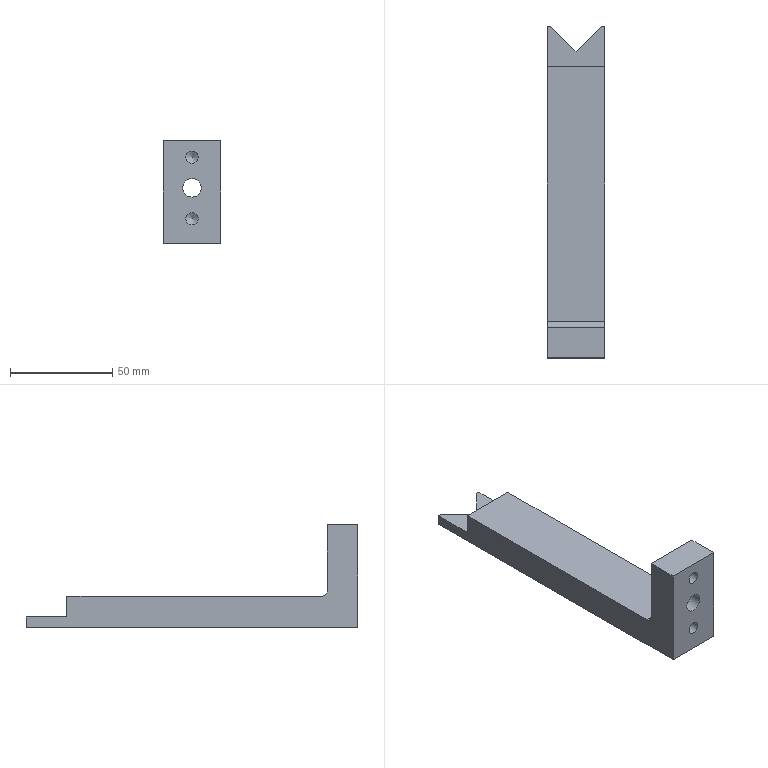Part | NX | features BREP 1 | 1 solid | 23 faces | box 28 x 162 x 50 mm | volume 74568 mm3 | plane 13 | cylinder 6 | cone 4 | commonest cylinder face diameters 6 x3 3.3 x2 9 x1
STEP:
#1=CARTESIAN_POINT('',(-14.,61.,7.5));
#2=VERTEX_POINT('',#1);
#3=CARTESIAN_POINT('',(-14.,-63.,7.5));
#4=VERTEX_POINT('',#3);
#5=CARTESIAN_POINT('',(-14.,-81.,7.5));
#6=DIRECTION('',(0.,-1.,0.));
#7=VECTOR('',#6,1000.);
#8=LINE('',#5,#7);
#9=EDGE_CURVE('',#2,#4,#8,.T.);
#10=ORIENTED_EDGE('',*,*,#9,.T.);
#11=CARTESIAN_POINT('',(14.,-63.,7.5));
#12=VERTEX_POINT('',#11);
#13=CARTESIAN_POINT('',(0.,-63.,7.5));
#14=DIRECTION('',(1.,0.,0.));
#15=VECTOR('',#14,1000.);
#16=LINE('',#13,#15);
#17=EDGE_CURVE('',#4,#12,#16,.T.);
#18=ORIENTED_EDGE('',*,*,#17,.T.);
#19=CARTESIAN_POINT('',(14.,61.,7.5));
#20=VERTEX_POINT('',#19);
#21=CARTESIAN_POINT('',(14.,-81.,7.5));
#22=DIRECTION('',(0.,1.,0.));
#23=VECTOR('',#22,1000.);
#24=LINE('',#21,#23);
#25=EDGE_CURVE('',#12,#20,#24,.T.);
#26=ORIENTED_EDGE('',*,*,#25,.T.);
#27=CARTESIAN_POINT('',(36.361,61.,7.5));
#28=DIRECTION('',(-1.,0.,0.));
#29=VECTOR('',#28,1000.);
#30=LINE('',#27,#29);
#31=EDGE_CURVE('',#20,#2,#30,.T.);
#32=ORIENTED_EDGE('',*,*,#31,.T.);
#33=EDGE_LOOP('',(#10,#18,#26,#32));
#34=FACE_BOUND('',#33,.T.);
#35=CARTESIAN_POINT('',(0.,0.,7.5));
#36=DIRECTION('',(0.,0.,-1.));
#37=DIRECTION('',(1.,0.,0.));
#38=AXIS2_PLACEMENT_3D('',#35,#36,#37);
#39=PLANE('',#38);
#40=ADVANCED_FACE('',(#34),#39,.F.);
#41=CARTESIAN_POINT('',(-14.,81.,-2.5));
#42=VERTEX_POINT('',#41);
#43=CARTESIAN_POINT('',(-14.,81.,-7.5));
#44=VERTEX_POINT('',#43);
#45=CARTESIAN_POINT('',(-14.,81.,7.5));
#46=DIRECTION('',(0.,0.,-1.));
#47=VECTOR('',#46,1000.);
#48=LINE('',#45,#47);
#49=EDGE_CURVE('',#42,#44,#48,.T.);
#50=ORIENTED_EDGE('',*,*,#49,.F.);
#51=CARTESIAN_POINT('',(-12.5,81.,-2.5));
#52=VERTEX_POINT('',#51);
#53=CARTESIAN_POINT('',(36.361,81.,-2.5));
#54=DIRECTION('',(-1.,0.,0.));
#55=VECTOR('',#54,1000.);
#56=LINE('',#53,#55);
#57=EDGE_CURVE('',#52,#42,#56,.T.);
#58=ORIENTED_EDGE('',*,*,#57,.F.);
#59=CARTESIAN_POINT('',(-12.5,81.,-7.5));
#60=VERTEX_POINT('',#59);
#61=CARTESIAN_POINT('',(-12.5,81.,35.451));
#62=DIRECTION('',(0.,0.,-1.));
#63=VECTOR('',#62,1000.);
#64=LINE('',#61,#63);
#65=EDGE_CURVE('',#52,#60,#64,.T.);
#66=ORIENTED_EDGE('',*,*,#65,.T.);
#67=CARTESIAN_POINT('',(-14.,81.,-7.5));
#68=DIRECTION('',(-1.,0.,0.));
#69=VECTOR('',#68,1000.);
#70=LINE('',#67,#69);
#71=EDGE_CURVE('',#60,#44,#70,.T.);
#72=ORIENTED_EDGE('',*,*,#71,.T.);
#73=EDGE_LOOP('',(#50,#58,#66,#72));
#74=FACE_BOUND('',#73,.T.);
#75=CARTESIAN_POINT('',(-14.,81.,7.5));
#76=DIRECTION('',(0.,-1.,0.));
#77=DIRECTION('',(0.,0.,1.));
#78=AXIS2_PLACEMENT_3D('',#75,#76,#77);
#79=PLANE('',#78);
#80=ADVANCED_FACE('',(#74),#79,.F.);
#81=CARTESIAN_POINT('',(14.,34.,-1.65));
#82=VERTEX_POINT('',#81);
#83=CARTESIAN_POINT('',(14.,34.,0.));
#84=DIRECTION('',(1.,0.,0.));
#85=DIRECTION('',(0.,0.,-1.));
#86=AXIS2_PLACEMENT_3D('',#83,#84,#85);
#87=CIRCLE('',#86,1.65);
#88=EDGE_CURVE('',#82,#82,#87,.T.);
#89=ORIENTED_EDGE('',*,*,#88,.F.);
#90=EDGE_LOOP('',(#89));
#91=FACE_BOUND('',#90,.T.);
#92=CARTESIAN_POINT('',(14.,24.,-1.65));
#93=VERTEX_POINT('',#92);
#94=CARTESIAN_POINT('',(14.,24.,0.));
#95=DIRECTION('',(1.,0.,0.));
#96=DIRECTION('',(0.,0.,-1.));
#97=AXIS2_PLACEMENT_3D('',#94,#95,#96);
#98=CIRCLE('',#97,1.65);
#99=EDGE_CURVE('',#93,#93,#98,.T.);
#100=ORIENTED_EDGE('',*,*,#99,.F.);
#101=EDGE_LOOP('',(#100));
#102=FACE_BOUND('',#101,.T.);
#103=CARTESIAN_POINT('',(14.,61.,-2.5));
#104=VERTEX_POINT('',#103);
#105=CARTESIAN_POINT('',(14.,81.,-2.5));
#106=VERTEX_POINT('',#105);
#107=CARTESIAN_POINT('',(14.,61.,-2.5));
#108=DIRECTION('',(0.,1.,0.));
#109=VECTOR('',#108,1000.);
#110=LINE('',#107,#109);
#111=EDGE_CURVE('',#104,#106,#110,.T.);
#112=ORIENTED_EDGE('',*,*,#111,.F.);
#113=CARTESIAN_POINT('',(14.,61.,7.5));
#114=DIRECTION('',(0.,0.,-1.));
#115=VECTOR('',#114,1000.);
#116=LINE('',#113,#115);
#117=EDGE_CURVE('',#20,#104,#116,.T.);
#118=ORIENTED_EDGE('',*,*,#117,.F.);
#119=ORIENTED_EDGE('',*,*,#25,.F.);
#120=CARTESIAN_POINT('',(14.,-66.,10.5));
#121=VERTEX_POINT('',#120);
#122=CARTESIAN_POINT('',(14.,-63.,10.5));
#123=DIRECTION('',(-1.,0.,0.));
#124=DIRECTION('',(0.,0.,1.));
#125=AXIS2_PLACEMENT_3D('',#122,#123,#124);
#126=CIRCLE('',#125,3.);
#127=EDGE_CURVE('',#12,#121,#126,.T.);
#128=ORIENTED_EDGE('',*,*,#127,.T.);
#129=CARTESIAN_POINT('',(14.,-66.,42.5));
#130=VERTEX_POINT('',#129);
#131=CARTESIAN_POINT('',(14.,-66.,7.5));
#132=DIRECTION('',(0.,0.,1.));
#133=VECTOR('',#132,1000.);
#134=LINE('',#131,#133);
#135=EDGE_CURVE('',#121,#130,#134,.T.);
#136=ORIENTED_EDGE('',*,*,#135,.T.);
#137=CARTESIAN_POINT('',(14.,-81.,42.5));
#138=VERTEX_POINT('',#137);
#139=CARTESIAN_POINT('',(14.,-81.,42.5));
#140=DIRECTION('',(0.,-1.,0.));
#141=VECTOR('',#140,1000.);
#142=LINE('',#139,#141);
#143=EDGE_CURVE('',#130,#138,#142,.T.);
#144=ORIENTED_EDGE('',*,*,#143,.T.);
#145=CARTESIAN_POINT('',(14.,-81.,-7.5));
#146=VERTEX_POINT('',#145);
#147=CARTESIAN_POINT('',(14.,-81.,7.5));
#148=DIRECTION('',(0.,0.,-1.));
#149=VECTOR('',#148,1000.);
#150=LINE('',#147,#149);
#151=EDGE_CURVE('',#138,#146,#150,.T.);
#152=ORIENTED_EDGE('',*,*,#151,.T.);
#153=CARTESIAN_POINT('',(14.,81.,-7.5));
#154=VERTEX_POINT('',#153);
#155=CARTESIAN_POINT('',(14.,-81.,-7.5));
#156=DIRECTION('',(0.,1.,0.));
#157=VECTOR('',#156,1000.);
#158=LINE('',#155,#157);
#159=EDGE_CURVE('',#146,#154,#158,.T.);
#160=ORIENTED_EDGE('',*,*,#159,.T.);
#161=CARTESIAN_POINT('',(14.,81.,7.5));
#162=DIRECTION('',(0.,0.,-1.));
#163=VECTOR('',#162,1000.);
#164=LINE('',#161,#163);
#165=EDGE_CURVE('',#106,#154,#164,.T.);
#166=ORIENTED_EDGE('',*,*,#165,.F.);
#167=EDGE_LOOP('',(#112,#118,#119,#128,#136,#144,#152,#160,#166));
#168=FACE_BOUND('',#167,.T.);
#169=CARTESIAN_POINT('',(14.,-81.,7.5));
#170=DIRECTION('',(-1.,0.,0.));
#171=DIRECTION('',(0.,0.,-1.));
#172=AXIS2_PLACEMENT_3D('',#169,#170,#171);
#173=PLANE('',#172);
#174=ADVANCED_FACE('',(#91,#102,#168),#173,.F.);
#175=CARTESIAN_POINT('',(12.5,81.,-2.5));
#176=VERTEX_POINT('',#175);
#177=CARTESIAN_POINT('',(12.5,81.,-7.5));
#178=VERTEX_POINT('',#177);
#179=CARTESIAN_POINT('',(12.5,81.,35.451));
#180=DIRECTION('',(0.,0.,-1.));
#181=VECTOR('',#180,1000.);
#182=LINE('',#179,#181);
#183=EDGE_CURVE('',#176,#178,#182,.T.);
#184=ORIENTED_EDGE('',*,*,#183,.F.);
#185=CARTESIAN_POINT('',(36.361,81.,-2.5));
#186=DIRECTION('',(-1.,0.,0.));
#187=VECTOR('',#186,1000.);
#188=LINE('',#185,#187);
#189=EDGE_CURVE('',#106,#176,#188,.T.);
#190=ORIENTED_EDGE('',*,*,#189,.F.);
#191=ORIENTED_EDGE('',*,*,#165,.T.);
#192=CARTESIAN_POINT('',(-14.,81.,-7.5));
#193=DIRECTION('',(-1.,0.,0.));
#194=VECTOR('',#193,1000.);
#195=LINE('',#192,#194);
#196=EDGE_CURVE('',#154,#178,#195,.T.);
#197=ORIENTED_EDGE('',*,*,#196,.T.);
#198=EDGE_LOOP('',(#184,#190,#191,#197));
#199=FACE_BOUND('',#198,.T.);
#200=CARTESIAN_POINT('',(-14.,81.,7.5));
#201=DIRECTION('',(0.,-1.,0.));
#202=DIRECTION('',(0.,0.,1.));
#203=AXIS2_PLACEMENT_3D('',#200,#201,#202);
#204=PLANE('',#203);
#205=ADVANCED_FACE('',(#199),#204,.F.);
#206=ORIENTED_EDGE('',*,*,#9,.F.);
#207=CARTESIAN_POINT('',(-14.,61.,-2.5));
#208=VERTEX_POINT('',#207);
#209=CARTESIAN_POINT('',(-14.,61.,7.5));
#210=DIRECTION('',(0.,0.,1.));
#211=VECTOR('',#210,1000.);
#212=LINE('',#209,#211);
#213=EDGE_CURVE('',#208,#2,#212,.T.);
#214=ORIENTED_EDGE('',*,*,#213,.F.);
#215=CARTESIAN_POINT('',(-14.,61.,-2.5));
#216=DIRECTION('',(0.,-1.,0.));
#217=VECTOR('',#216,1000.);
#218=LINE('',#215,#217);
#219=EDGE_CURVE('',#42,#208,#218,.T.);
#220=ORIENTED_EDGE('',*,*,#219,.F.);
#221=ORIENTED_EDGE('',*,*,#49,.T.);
#222=CARTESIAN_POINT('',(-14.,-81.,-7.5));
#223=VERTEX_POINT('',#222);
#224=CARTESIAN_POINT('',(-14.,-81.,-7.5));
#225=DIRECTION('',(0.,-1.,0.));
#226=VECTOR('',#225,1000.);
#227=LINE('',#224,#226);
#228=EDGE_CURVE('',#44,#223,#227,.T.);
#229=ORIENTED_EDGE('',*,*,#228,.T.);
#230=CARTESIAN_POINT('',(-14.,-81.,42.5));
#231=VERTEX_POINT('',#230);
#232=CARTESIAN_POINT('',(-14.,-81.,7.5));
#233=DIRECTION('',(0.,0.,-1.));
#234=VECTOR('',#233,1000.);
#235=LINE('',#232,#234);
#236=EDGE_CURVE('',#231,#223,#235,.T.);
#237=ORIENTED_EDGE('',*,*,#236,.F.);
#238=CARTESIAN_POINT('',(-14.,-66.,42.5));
#239=VERTEX_POINT('',#238);
#240=CARTESIAN_POINT('',(-14.,-81.,42.5));
#241=DIRECTION('',(0.,1.,0.));
#242=VECTOR('',#241,1000.);
#243=LINE('',#240,#242);
#244=EDGE_CURVE('',#231,#239,#243,.T.);
#245=ORIENTED_EDGE('',*,*,#244,.T.);
#246=CARTESIAN_POINT('',(-14.,-66.,10.5));
#247=VERTEX_POINT('',#246);
#248=CARTESIAN_POINT('',(-14.,-66.,7.5));
#249=DIRECTION('',(0.,0.,-1.));
#250=VECTOR('',#249,1000.);
#251=LINE('',#248,#250);
#252=EDGE_CURVE('',#239,#247,#251,.T.);
#253=ORIENTED_EDGE('',*,*,#252,.T.);
#254=CARTESIAN_POINT('',(-14.,-63.,10.5));
#255=DIRECTION('',(1.,0.,0.));
#256=DIRECTION('',(0.,0.,-1.));
#257=AXIS2_PLACEMENT_3D('',#254,#255,#256);
#258=CIRCLE('',#257,3.);
#259=EDGE_CURVE('',#247,#4,#258,.T.);
#260=ORIENTED_EDGE('',*,*,#259,.T.);
#261=EDGE_LOOP('',(#206,#214,#220,#221,#229,#237,#245,#253,#260));
#262=FACE_BOUND('',#261,.T.);
#263=CARTESIAN_POINT('',(-14.,-81.,7.5));
#264=DIRECTION('',(1.,0.,0.));
#265=DIRECTION('',(0.,0.,1.));
#266=AXIS2_PLACEMENT_3D('',#263,#264,#265);
#267=PLANE('',#266);
#268=ADVANCED_FACE('',(#262),#267,.F.);
#269=CARTESIAN_POINT('',(0.,-81.,24.));
#270=VERTEX_POINT('',#269);
#271=CARTESIAN_POINT('',(0.,-81.,19.5));
#272=DIRECTION('',(0.,1.,0.));
#273=DIRECTION('',(0.,0.,1.));
#274=AXIS2_PLACEMENT_3D('',#271,#272,#273);
#275=CIRCLE('',#274,4.5);
#276=EDGE_CURVE('',#270,#270,#275,.T.);
#277=ORIENTED_EDGE('',*,*,#276,.T.);
#278=EDGE_LOOP('',(#277));
#279=FACE_BOUND('',#278,.T.);
#280=CARTESIAN_POINT('',(0.,-81.,31.5));
#281=VERTEX_POINT('',#280);
#282=CARTESIAN_POINT('',(0.,-81.,34.5));
#283=DIRECTION('',(0.,-1.,0.));
#284=DIRECTION('',(0.,0.,-1.));
#285=AXIS2_PLACEMENT_3D('',#282,#283,#284);
#286=CIRCLE('',#285,3.);
#287=EDGE_CURVE('',#281,#281,#286,.T.);
#288=ORIENTED_EDGE('',*,*,#287,.F.);
#289=EDGE_LOOP('',(#288));
#290=FACE_BOUND('',#289,.T.);
#291=CARTESIAN_POINT('',(0.,-81.,1.5));
#292=VERTEX_POINT('',#291);
#293=CARTESIAN_POINT('',(0.,-81.,4.5));
#294=DIRECTION('',(0.,-1.,0.));
#295=DIRECTION('',(0.,0.,-1.));
#296=AXIS2_PLACEMENT_3D('',#293,#294,#295);
#297=CIRCLE('',#296,3.);
#298=EDGE_CURVE('',#292,#292,#297,.T.);
#299=ORIENTED_EDGE('',*,*,#298,.F.);
#300=EDGE_LOOP('',(#299));
#301=FACE_BOUND('',#300,.T.);
#302=CARTESIAN_POINT('',(-14.,-81.,-7.5));
#303=DIRECTION('',(1.,0.,0.));
#304=VECTOR('',#303,1000.);
#305=LINE('',#302,#304);
#306=EDGE_CURVE('',#223,#146,#305,.T.);
#307=ORIENTED_EDGE('',*,*,#306,.T.);
#308=ORIENTED_EDGE('',*,*,#151,.F.);
#309=CARTESIAN_POINT('',(52.079,-81.,42.5));
#310=DIRECTION('',(-1.,0.,0.));
#311=VECTOR('',#310,1000.);
#312=LINE('',#309,#311);
#313=EDGE_CURVE('',#138,#231,#312,.T.);
#314=ORIENTED_EDGE('',*,*,#313,.T.);
#315=ORIENTED_EDGE('',*,*,#236,.T.);
#316=EDGE_LOOP('',(#307,#308,#314,#315));
#317=FACE_BOUND('',#316,.T.);
#318=CARTESIAN_POINT('',(-14.,-81.,7.5));
#319=DIRECTION('',(0.,1.,0.));
#320=DIRECTION('',(0.,0.,-1.));
#321=AXIS2_PLACEMENT_3D('',#318,#319,#320);
#322=PLANE('',#321);
#323=ADVANCED_FACE('',(#279,#290,#301,#317),#322,.F.);
#324=CARTESIAN_POINT('',(0.,68.5,-7.5));
#325=VERTEX_POINT('',#324);
#326=CARTESIAN_POINT('',(0.,68.5,-7.5));
#327=DIRECTION('',(-0.7071,0.7071,0.));
#328=VECTOR('',#327,1000.);
#329=LINE('',#326,#328);
#330=EDGE_CURVE('',#325,#60,#329,.T.);
#331=ORIENTED_EDGE('',*,*,#330,.F.);
#332=CARTESIAN_POINT('',(12.5,81.,-7.5));
#333=DIRECTION('',(-0.7071,-0.7071,0.));
#334=VECTOR('',#333,1000.);
#335=LINE('',#332,#334);
#336=EDGE_CURVE('',#178,#325,#335,.T.);
#337=ORIENTED_EDGE('',*,*,#336,.F.);
#338=ORIENTED_EDGE('',*,*,#196,.F.);
#339=ORIENTED_EDGE('',*,*,#159,.F.);
#340=ORIENTED_EDGE('',*,*,#306,.F.);
#341=ORIENTED_EDGE('',*,*,#228,.F.);
#342=ORIENTED_EDGE('',*,*,#71,.F.);
#343=EDGE_LOOP('',(#331,#337,#338,#339,#340,#341,#342));
#344=FACE_BOUND('',#343,.T.);
#345=CARTESIAN_POINT('',(0.,0.,-7.5));
#346=DIRECTION('',(0.,0.,-1.));
#347=DIRECTION('',(1.,0.,0.));
#348=AXIS2_PLACEMENT_3D('',#345,#346,#347);
#349=PLANE('',#348);
#350=ADVANCED_FACE('',(#344),#349,.T.);
#351=ORIENTED_EDGE('',*,*,#65,.F.);
#352=CARTESIAN_POINT('',(0.,68.5,-2.5));
#353=VERTEX_POINT('',#352);
#354=CARTESIAN_POINT('',(0.,68.5,-2.5));
#355=DIRECTION('',(0.7071,-0.7071,0.));
#356=VECTOR('',#355,1000.);
#357=LINE('',#354,#356);
#358=EDGE_CURVE('',#52,#353,#357,.T.);
#359=ORIENTED_EDGE('',*,*,#358,.T.);
#360=CARTESIAN_POINT('',(0.,68.5,35.451));
#361=DIRECTION('',(0.,0.,-1.));
#362=VECTOR('',#361,1000.);
#363=LINE('',#360,#362);
#364=EDGE_CURVE('',#353,#325,#363,.T.);
#365=ORIENTED_EDGE('',*,*,#364,.T.);
#366=ORIENTED_EDGE('',*,*,#330,.T.);
#367=EDGE_LOOP('',(#351,#359,#365,#366));
#368=FACE_BOUND('',#367,.T.);
#369=CARTESIAN_POINT('',(0.,68.5,35.451));
#370=DIRECTION('',(-0.7071,-0.7071,0.));
#371=DIRECTION('',(-0.7071,0.7071,0.));
#372=AXIS2_PLACEMENT_3D('',#369,#370,#371);
#373=PLANE('',#372);
#374=ADVANCED_FACE('',(#368),#373,.F.);
#375=ORIENTED_EDGE('',*,*,#364,.F.);
#376=CARTESIAN_POINT('',(12.5,81.,-2.5));
#377=DIRECTION('',(0.7071,0.7071,0.));
#378=VECTOR('',#377,1000.);
#379=LINE('',#376,#378);
#380=EDGE_CURVE('',#353,#176,#379,.T.);
#381=ORIENTED_EDGE('',*,*,#380,.T.);
#382=ORIENTED_EDGE('',*,*,#183,.T.);
#383=ORIENTED_EDGE('',*,*,#336,.T.);
#384=EDGE_LOOP('',(#375,#381,#382,#383));
#385=FACE_BOUND('',#384,.T.);
#386=CARTESIAN_POINT('',(12.5,81.,35.451));
#387=DIRECTION('',(0.7071,-0.7071,0.));
#388=DIRECTION('',(-0.7071,-0.7071,0.));
#389=AXIS2_PLACEMENT_3D('',#386,#387,#388);
#390=PLANE('',#389);
#391=ADVANCED_FACE('',(#385),#390,.F.);
#392=ORIENTED_EDGE('',*,*,#57,.T.);
#393=ORIENTED_EDGE('',*,*,#219,.T.);
#394=CARTESIAN_POINT('',(36.361,61.,-2.5));
#395=DIRECTION('',(-1.,0.,0.));
#396=VECTOR('',#395,1000.);
#397=LINE('',#394,#396);
#398=EDGE_CURVE('',#104,#208,#397,.T.);
#399=ORIENTED_EDGE('',*,*,#398,.F.);
#400=ORIENTED_EDGE('',*,*,#111,.T.);
#401=ORIENTED_EDGE('',*,*,#189,.T.);
#402=ORIENTED_EDGE('',*,*,#380,.F.);
#403=ORIENTED_EDGE('',*,*,#358,.F.);
#404=EDGE_LOOP('',(#392,#393,#399,#400,#401,#402,#403));
#405=FACE_BOUND('',#404,.T.);
#406=CARTESIAN_POINT('',(36.361,61.,-2.5));
#407=DIRECTION('',(0.,0.,-1.));
#408=DIRECTION('',(0.,-1.,0.));
#409=AXIS2_PLACEMENT_3D('',#406,#407,#408);
#410=PLANE('',#409);
#411=ADVANCED_FACE('',(#405),#410,.F.);
#412=ORIENTED_EDGE('',*,*,#117,.T.);
#413=ORIENTED_EDGE('',*,*,#398,.T.);
#414=ORIENTED_EDGE('',*,*,#213,.T.);
#415=ORIENTED_EDGE('',*,*,#31,.F.);
#416=EDGE_LOOP('',(#412,#413,#414,#415));
#417=FACE_BOUND('',#416,.T.);
#418=CARTESIAN_POINT('',(36.361,61.,7.5));
#419=DIRECTION('',(0.,-1.,0.));
#420=DIRECTION('',(0.,0.,1.));
#421=AXIS2_PLACEMENT_3D('',#418,#419,#420);
#422=PLANE('',#421);
#423=ADVANCED_FACE('',(#417),#422,.F.);
#424=CARTESIAN_POINT('',(0.,-66.,24.));
#425=VERTEX_POINT('',#424);
#426=CARTESIAN_POINT('',(0.,-66.,19.5));
#427=DIRECTION('',(0.,1.,0.));
#428=DIRECTION('',(0.,0.,1.));
#429=AXIS2_PLACEMENT_3D('',#426,#427,#428);
#430=CIRCLE('',#429,4.5);
#431=EDGE_CURVE('',#425,#425,#430,.T.);
#432=ORIENTED_EDGE('',*,*,#431,.F.);
#433=EDGE_LOOP('',(#432));
#434=FACE_BOUND('',#433,.T.);
#435=ORIENTED_EDGE('',*,*,#135,.F.);
#436=CARTESIAN_POINT('',(52.079,-66.,10.5));
#437=DIRECTION('',(-1.,0.,0.));
#438=VECTOR('',#437,1000.);
#439=LINE('',#436,#438);
#440=EDGE_CURVE('',#121,#247,#439,.T.);
#441=ORIENTED_EDGE('',*,*,#440,.T.);
#442=ORIENTED_EDGE('',*,*,#252,.F.);
#443=CARTESIAN_POINT('',(52.079,-66.,42.5));
#444=DIRECTION('',(-1.,0.,0.));
#445=VECTOR('',#444,1000.);
#446=LINE('',#443,#445);
#447=EDGE_CURVE('',#130,#239,#446,.T.);
#448=ORIENTED_EDGE('',*,*,#447,.F.);
#449=EDGE_LOOP('',(#435,#441,#442,#448));
#450=FACE_BOUND('',#449,.T.);
#451=CARTESIAN_POINT('',(52.079,-66.,7.5));
#452=DIRECTION('',(0.,1.,0.));
#453=DIRECTION('',(0.,0.,-1.));
#454=AXIS2_PLACEMENT_3D('',#451,#452,#453);
#455=PLANE('',#454);
#456=ADVANCED_FACE('',(#434,#450),#455,.T.);
#457=ORIENTED_EDGE('',*,*,#143,.F.);
#458=ORIENTED_EDGE('',*,*,#447,.T.);
#459=ORIENTED_EDGE('',*,*,#244,.F.);
#460=ORIENTED_EDGE('',*,*,#313,.F.);
#461=EDGE_LOOP('',(#457,#458,#459,#460));
#462=FACE_BOUND('',#461,.T.);
#463=CARTESIAN_POINT('',(52.079,-81.,42.5));
#464=DIRECTION('',(0.,0.,1.));
#465=DIRECTION('',(-1.,0.,0.));
#466=AXIS2_PLACEMENT_3D('',#463,#464,#465);
#467=PLANE('',#466);
#468=ADVANCED_FACE('',(#462),#467,.T.);
#469=CARTESIAN_POINT('',(0.,-67.197,4.5));
#470=VERTEX_POINT('',#469);
#471=VERTEX_LOOP('',#470);
#472=FACE_BOUND('',#471,.T.);
#473=CARTESIAN_POINT('',(0.,-69.,1.5));
#474=VERTEX_POINT('',#473);
#475=CARTESIAN_POINT('',(0.,-69.,4.5));
#476=DIRECTION('',(0.,-1.,0.));
#477=DIRECTION('',(0.,0.,-1.));
#478=AXIS2_PLACEMENT_3D('',#475,#476,#477);
#479=CIRCLE('',#478,3.);
#480=EDGE_CURVE('',#474,#474,#479,.T.);
#481=ORIENTED_EDGE('',*,*,#480,.T.);
#482=EDGE_LOOP('',(#481));
#483=FACE_BOUND('',#482,.T.);
#484=CARTESIAN_POINT('',(0.,-69.,4.5));
#485=DIRECTION('',(0.,-1.,0.));
#486=DIRECTION('',(0.,0.,1.));
#487=AXIS2_PLACEMENT_3D('',#484,#485,#486);
#488=CONICAL_SURFACE('',#487,3.,1.03);
#489=ADVANCED_FACE('',(#472,#483),#488,.F.);
#490=ORIENTED_EDGE('',*,*,#480,.F.);
#491=EDGE_LOOP('',(#490));
#492=FACE_BOUND('',#491,.T.);
#493=ORIENTED_EDGE('',*,*,#298,.T.);
#494=EDGE_LOOP('',(#493));
#495=FACE_BOUND('',#494,.T.);
#496=CARTESIAN_POINT('',(0.,-81.,4.5));
#497=DIRECTION('',(0.,-1.,0.));
#498=DIRECTION('',(0.,0.,1.));
#499=AXIS2_PLACEMENT_3D('',#496,#497,#498);
#500=CYLINDRICAL_SURFACE('',#499,3.);
#501=ADVANCED_FACE('',(#492,#495),#500,.F.);
#502=CARTESIAN_POINT('',(0.,-67.197,34.5));
#503=VERTEX_POINT('',#502);
#504=VERTEX_LOOP('',#503);
#505=FACE_BOUND('',#504,.T.);
#506=CARTESIAN_POINT('',(0.,-69.,31.5));
#507=VERTEX_POINT('',#506);
#508=CARTESIAN_POINT('',(0.,-69.,34.5));
#509=DIRECTION('',(0.,-1.,0.));
#510=DIRECTION('',(0.,0.,-1.));
#511=AXIS2_PLACEMENT_3D('',#508,#509,#510);
#512=CIRCLE('',#511,3.);
#513=EDGE_CURVE('',#507,#507,#512,.T.);
#514=ORIENTED_EDGE('',*,*,#513,.T.);
#515=EDGE_LOOP('',(#514));
#516=FACE_BOUND('',#515,.T.);
#517=CARTESIAN_POINT('',(0.,-69.,34.5));
#518=DIRECTION('',(0.,-1.,0.));
#519=DIRECTION('',(0.,0.,1.));
#520=AXIS2_PLACEMENT_3D('',#517,#518,#519);
#521=CONICAL_SURFACE('',#520,3.,1.03);
#522=ADVANCED_FACE('',(#505,#516),#521,.F.);
#523=ORIENTED_EDGE('',*,*,#513,.F.);
#524=EDGE_LOOP('',(#523));
#525=FACE_BOUND('',#524,.T.);
#526=ORIENTED_EDGE('',*,*,#287,.T.);
#527=EDGE_LOOP('',(#526));
#528=FACE_BOUND('',#527,.T.);
#529=CARTESIAN_POINT('',(0.,-81.,34.5));
#530=DIRECTION('',(0.,-1.,0.));
#531=DIRECTION('',(0.,0.,1.));
#532=AXIS2_PLACEMENT_3D('',#529,#530,#531);
#533=CYLINDRICAL_SURFACE('',#532,3.);
#534=ADVANCED_FACE('',(#525,#528),#533,.F.);
#535=ORIENTED_EDGE('',*,*,#276,.F.);
#536=EDGE_LOOP('',(#535));
#537=FACE_BOUND('',#536,.T.);
#538=ORIENTED_EDGE('',*,*,#431,.T.);
#539=EDGE_LOOP('',(#538));
#540=FACE_BOUND('',#539,.T.);
#541=CARTESIAN_POINT('',(0.,-66.,19.5));
#542=DIRECTION('',(0.,1.,0.));
#543=DIRECTION('',(0.,0.,-1.));
#544=AXIS2_PLACEMENT_3D('',#541,#542,#543);
#545=CYLINDRICAL_SURFACE('',#544,4.5);
#546=ADVANCED_FACE('',(#537,#540),#545,.F.);
#547=ORIENTED_EDGE('',*,*,#127,.F.);
#548=ORIENTED_EDGE('',*,*,#17,.F.);
#549=ORIENTED_EDGE('',*,*,#259,.F.);
#550=ORIENTED_EDGE('',*,*,#440,.F.);
#551=EDGE_LOOP('',(#547,#548,#549,#550));
#552=FACE_BOUND('',#551,.T.);
#553=CARTESIAN_POINT('',(52.079,-63.,10.5));
#554=DIRECTION('',(-1.,0.,0.));
#555=DIRECTION('',(0.,0.,-1.));
#556=AXIS2_PLACEMENT_3D('',#553,#554,#555);
#557=CYLINDRICAL_SURFACE('',#556,3.);
#558=ADVANCED_FACE('',(#552),#557,.F.);
#559=CARTESIAN_POINT('',(2.909,24.,0.));
#560=VERTEX_POINT('',#559);
#561=VERTEX_LOOP('',#560);
#562=FACE_BOUND('',#561,.T.);
#563=CARTESIAN_POINT('',(3.9,24.,-1.65));
#564=VERTEX_POINT('',#563);
#565=CARTESIAN_POINT('',(3.9,24.,0.));
#566=DIRECTION('',(1.,0.,0.));
#567=DIRECTION('',(0.,0.,-1.));
#568=AXIS2_PLACEMENT_3D('',#565,#566,#567);
#569=CIRCLE('',#568,1.65);
#570=EDGE_CURVE('',#564,#564,#569,.T.);
#571=ORIENTED_EDGE('',*,*,#570,.T.);
#572=EDGE_LOOP('',(#571));
#573=FACE_BOUND('',#572,.T.);
#574=CARTESIAN_POINT('',(3.9,24.,0.));
#575=DIRECTION('',(1.,0.,0.));
#576=DIRECTION('',(0.,0.,1.));
#577=AXIS2_PLACEMENT_3D('',#574,#575,#576);
#578=CONICAL_SURFACE('',#577,1.65,1.03);
#579=ADVANCED_FACE('',(#562,#573),#578,.F.);
#580=ORIENTED_EDGE('',*,*,#570,.F.);
#581=EDGE_LOOP('',(#580));
#582=FACE_BOUND('',#581,.T.);
#583=ORIENTED_EDGE('',*,*,#99,.T.);
#584=EDGE_LOOP('',(#583));
#585=FACE_BOUND('',#584,.T.);
#586=CARTESIAN_POINT('',(14.,24.,0.));
#587=DIRECTION('',(1.,0.,0.));
#588=DIRECTION('',(0.,0.,1.));
#589=AXIS2_PLACEMENT_3D('',#586,#587,#588);
#590=CYLINDRICAL_SURFACE('',#589,1.65);
#591=ADVANCED_FACE('',(#582,#585),#590,.F.);
#592=CARTESIAN_POINT('',(2.909,34.,0.));
#593=VERTEX_POINT('',#592);
#594=VERTEX_LOOP('',#593);
#595=FACE_BOUND('',#594,.T.);
#596=CARTESIAN_POINT('',(3.9,34.,-1.65));
#597=VERTEX_POINT('',#596);
#598=CARTESIAN_POINT('',(3.9,34.,0.));
#599=DIRECTION('',(1.,0.,0.));
#600=DIRECTION('',(0.,0.,-1.));
#601=AXIS2_PLACEMENT_3D('',#598,#599,#600);
#602=CIRCLE('',#601,1.65);
#603=EDGE_CURVE('',#597,#597,#602,.T.);
#604=ORIENTED_EDGE('',*,*,#603,.T.);
#605=EDGE_LOOP('',(#604));
#606=FACE_BOUND('',#605,.T.);
#607=CARTESIAN_POINT('',(3.9,34.,0.));
#608=DIRECTION('',(1.,0.,0.));
#609=DIRECTION('',(0.,0.,1.));
#610=AXIS2_PLACEMENT_3D('',#607,#608,#609);
#611=CONICAL_SURFACE('',#610,1.65,1.03);
#612=ADVANCED_FACE('',(#595,#606),#611,.F.);
#613=ORIENTED_EDGE('',*,*,#603,.F.);
#614=EDGE_LOOP('',(#613));
#615=FACE_BOUND('',#614,.T.);
#616=ORIENTED_EDGE('',*,*,#88,.T.);
#617=EDGE_LOOP('',(#616));
#618=FACE_BOUND('',#617,.T.);
#619=CARTESIAN_POINT('',(14.,34.,0.));
#620=DIRECTION('',(1.,0.,0.));
#621=DIRECTION('',(0.,0.,1.));
#622=AXIS2_PLACEMENT_3D('',#619,#620,#621);
#623=CYLINDRICAL_SURFACE('',#622,1.65);
#624=ADVANCED_FACE('',(#615,#618),#623,.F.);
#625=CLOSED_SHELL('',(#40,#80,#174,#205,#268,#323,#350,#374,#391,#411,#423,#456,#468,#489,#501,#522,#534,#546,#558,#579,#591,#612,#624));
#626=MANIFOLD_SOLID_BREP('',#625);
#627=(LENGTH_UNIT()NAMED_UNIT(*)SI_UNIT(.MILLI.,.METRE.));
#628=UNCERTAINTY_MEASURE_WITH_UNIT(LENGTH_MEASURE(0.00001),#627,'','');
#629=(NAMED_UNIT(*)PLANE_ANGLE_UNIT()SI_UNIT($,.RADIAN.));
#630=(NAMED_UNIT(*)SI_UNIT($,.STERADIAN.)SOLID_ANGLE_UNIT());
#631=(GEOMETRIC_REPRESENTATION_CONTEXT(3)GLOBAL_UNCERTAINTY_ASSIGNED_CONTEXT((#628))GLOBAL_UNIT_ASSIGNED_CONTEXT((#627,#629,#630))REPRESENTATION_CONTEXT('',''));
#632=ADVANCED_BREP_SHAPE_REPRESENTATION('',(#626),#631);